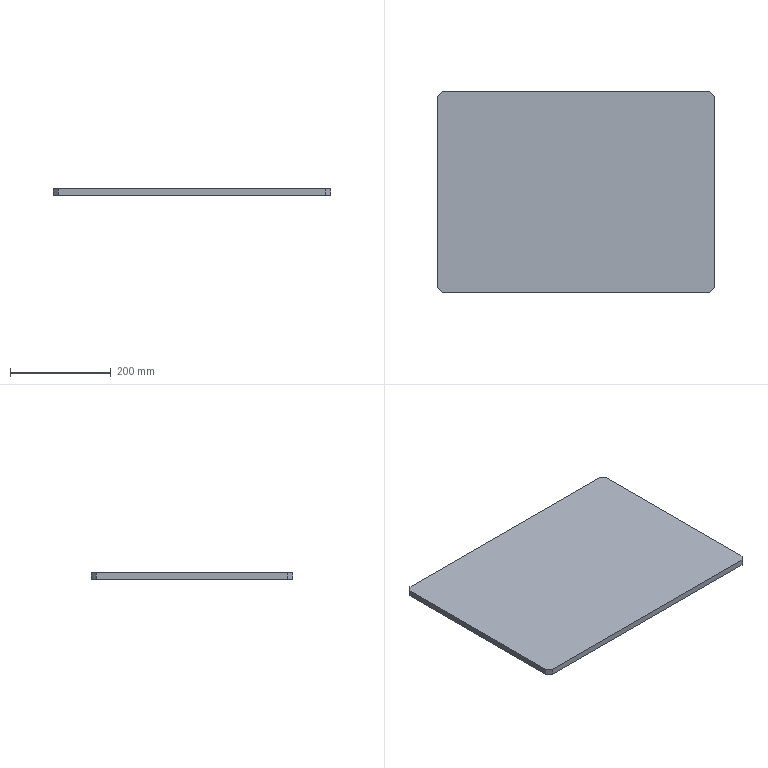Part | NX | features BREP 1 | 1 solid | 10 faces | box 550 x 400 x 12 mm | volume 2637600 mm3 | plane 10
STEP:
#1=CARTESIAN_POINT('',(308.,-205.,0.));
#2=VERTEX_POINT('',#1);
#3=CARTESIAN_POINT('',(308.,175.,0.));
#4=VERTEX_POINT('',#3);
#5=CARTESIAN_POINT('',(308.,-150.,0.));
#6=DIRECTION('',(0.,1.,0.));
#7=VECTOR('',#6,1000.);
#8=LINE('',#5,#7);
#9=EDGE_CURVE('',#2,#4,#8,.T.);
#10=ORIENTED_EDGE('',*,*,#9,.T.);
#11=CARTESIAN_POINT('',(308.,175.,12.));
#12=VERTEX_POINT('',#11);
#13=CARTESIAN_POINT('',(308.,175.,12.));
#14=DIRECTION('',(0.,0.,1.));
#15=VECTOR('',#14,1000.);
#16=LINE('',#13,#15);
#17=EDGE_CURVE('',#4,#12,#16,.T.);
#18=ORIENTED_EDGE('',*,*,#17,.T.);
#19=CARTESIAN_POINT('',(308.,-205.,12.));
#20=VERTEX_POINT('',#19);
#21=CARTESIAN_POINT('',(308.,-150.,12.));
#22=DIRECTION('',(0.,1.,0.));
#23=VECTOR('',#22,1000.);
#24=LINE('',#21,#23);
#25=EDGE_CURVE('',#20,#12,#24,.T.);
#26=ORIENTED_EDGE('',*,*,#25,.F.);
#27=CARTESIAN_POINT('',(308.,-205.,12.));
#28=DIRECTION('',(0.,0.,-1.));
#29=VECTOR('',#28,1000.);
#30=LINE('',#27,#29);
#31=EDGE_CURVE('',#20,#2,#30,.T.);
#32=ORIENTED_EDGE('',*,*,#31,.T.);
#33=EDGE_LOOP('',(#10,#18,#26,#32));
#34=FACE_BOUND('',#33,.T.);
#35=CARTESIAN_POINT('',(308.,-150.,12.));
#36=DIRECTION('',(-1.,0.,0.));
#37=DIRECTION('',(0.,0.,1.));
#38=AXIS2_PLACEMENT_3D('',#35,#36,#37);
#39=PLANE('',#38);
#40=ADVANCED_FACE('',(#34),#39,.F.);
#41=CARTESIAN_POINT('',(298.,185.,0.));
#42=VERTEX_POINT('',#41);
#43=CARTESIAN_POINT('',(-232.,185.,0.));
#44=VERTEX_POINT('',#43);
#45=CARTESIAN_POINT('',(-150.,185.,0.));
#46=DIRECTION('',(-1.,0.,0.));
#47=VECTOR('',#46,1000.);
#48=LINE('',#45,#47);
#49=EDGE_CURVE('',#42,#44,#48,.T.);
#50=ORIENTED_EDGE('',*,*,#49,.T.);
#51=CARTESIAN_POINT('',(-232.,185.,12.));
#52=VERTEX_POINT('',#51);
#53=CARTESIAN_POINT('',(-232.,185.,12.));
#54=DIRECTION('',(0.,0.,1.));
#55=VECTOR('',#54,1000.);
#56=LINE('',#53,#55);
#57=EDGE_CURVE('',#44,#52,#56,.T.);
#58=ORIENTED_EDGE('',*,*,#57,.T.);
#59=CARTESIAN_POINT('',(298.,185.,12.));
#60=VERTEX_POINT('',#59);
#61=CARTESIAN_POINT('',(-150.,185.,12.));
#62=DIRECTION('',(-1.,0.,0.));
#63=VECTOR('',#62,1000.);
#64=LINE('',#61,#63);
#65=EDGE_CURVE('',#60,#52,#64,.T.);
#66=ORIENTED_EDGE('',*,*,#65,.F.);
#67=CARTESIAN_POINT('',(298.,185.,12.));
#68=DIRECTION('',(0.,0.,-1.));
#69=VECTOR('',#68,1000.);
#70=LINE('',#67,#69);
#71=EDGE_CURVE('',#60,#42,#70,.T.);
#72=ORIENTED_EDGE('',*,*,#71,.T.);
#73=EDGE_LOOP('',(#50,#58,#66,#72));
#74=FACE_BOUND('',#73,.T.);
#75=CARTESIAN_POINT('',(-150.,185.,12.));
#76=DIRECTION('',(0.,-1.,0.));
#77=DIRECTION('',(0.,0.,-1.));
#78=AXIS2_PLACEMENT_3D('',#75,#76,#77);
#79=PLANE('',#78);
#80=ADVANCED_FACE('',(#74),#79,.F.);
#81=CARTESIAN_POINT('',(-242.,175.,12.));
#82=VERTEX_POINT('',#81);
#83=CARTESIAN_POINT('',(-242.,-205.,12.));
#84=VERTEX_POINT('',#83);
#85=CARTESIAN_POINT('',(-242.,-150.,12.));
#86=DIRECTION('',(0.,-1.,0.));
#87=VECTOR('',#86,1000.);
#88=LINE('',#85,#87);
#89=EDGE_CURVE('',#82,#84,#88,.T.);
#90=ORIENTED_EDGE('',*,*,#89,.F.);
#91=CARTESIAN_POINT('',(-242.,175.,0.));
#92=VERTEX_POINT('',#91);
#93=CARTESIAN_POINT('',(-242.,175.,12.));
#94=DIRECTION('',(0.,0.,-1.));
#95=VECTOR('',#94,1000.);
#96=LINE('',#93,#95);
#97=EDGE_CURVE('',#82,#92,#96,.T.);
#98=ORIENTED_EDGE('',*,*,#97,.T.);
#99=CARTESIAN_POINT('',(-242.,-205.,0.));
#100=VERTEX_POINT('',#99);
#101=CARTESIAN_POINT('',(-242.,-150.,0.));
#102=DIRECTION('',(0.,-1.,0.));
#103=VECTOR('',#102,1000.);
#104=LINE('',#101,#103);
#105=EDGE_CURVE('',#92,#100,#104,.T.);
#106=ORIENTED_EDGE('',*,*,#105,.T.);
#107=CARTESIAN_POINT('',(-242.,-205.,12.));
#108=DIRECTION('',(0.,0.,1.));
#109=VECTOR('',#108,1000.);
#110=LINE('',#107,#109);
#111=EDGE_CURVE('',#100,#84,#110,.T.);
#112=ORIENTED_EDGE('',*,*,#111,.T.);
#113=EDGE_LOOP('',(#90,#98,#106,#112));
#114=FACE_BOUND('',#113,.T.);
#115=CARTESIAN_POINT('',(-242.,-150.,12.));
#116=DIRECTION('',(1.,0.,0.));
#117=DIRECTION('',(0.,1.,0.));
#118=AXIS2_PLACEMENT_3D('',#115,#116,#117);
#119=PLANE('',#118);
#120=ADVANCED_FACE('',(#114),#119,.F.);
#121=CARTESIAN_POINT('',(-232.,-215.,0.));
#122=VERTEX_POINT('',#121);
#123=CARTESIAN_POINT('',(298.,-215.,0.));
#124=VERTEX_POINT('',#123);
#125=CARTESIAN_POINT('',(-150.,-215.,0.));
#126=DIRECTION('',(1.,0.,0.));
#127=VECTOR('',#126,1000.);
#128=LINE('',#125,#127);
#129=EDGE_CURVE('',#122,#124,#128,.T.);
#130=ORIENTED_EDGE('',*,*,#129,.T.);
#131=CARTESIAN_POINT('',(298.,-215.,12.));
#132=VERTEX_POINT('',#131);
#133=CARTESIAN_POINT('',(298.,-215.,12.));
#134=DIRECTION('',(0.,0.,1.));
#135=VECTOR('',#134,1000.);
#136=LINE('',#133,#135);
#137=EDGE_CURVE('',#124,#132,#136,.T.);
#138=ORIENTED_EDGE('',*,*,#137,.T.);
#139=CARTESIAN_POINT('',(-232.,-215.,12.));
#140=VERTEX_POINT('',#139);
#141=CARTESIAN_POINT('',(-150.,-215.,12.));
#142=DIRECTION('',(1.,0.,0.));
#143=VECTOR('',#142,1000.);
#144=LINE('',#141,#143);
#145=EDGE_CURVE('',#140,#132,#144,.T.);
#146=ORIENTED_EDGE('',*,*,#145,.F.);
#147=CARTESIAN_POINT('',(-232.,-215.,12.));
#148=DIRECTION('',(0.,0.,-1.));
#149=VECTOR('',#148,1000.);
#150=LINE('',#147,#149);
#151=EDGE_CURVE('',#140,#122,#150,.T.);
#152=ORIENTED_EDGE('',*,*,#151,.T.);
#153=EDGE_LOOP('',(#130,#138,#146,#152));
#154=FACE_BOUND('',#153,.T.);
#155=CARTESIAN_POINT('',(-150.,-215.,12.));
#156=DIRECTION('',(0.,1.,0.));
#157=DIRECTION('',(1.,0.,0.));
#158=AXIS2_PLACEMENT_3D('',#155,#156,#157);
#159=PLANE('',#158);
#160=ADVANCED_FACE('',(#154),#159,.F.);
#161=ORIENTED_EDGE('',*,*,#65,.T.);
#162=CARTESIAN_POINT('',(-242.,175.,12.));
#163=DIRECTION('',(-0.7071,-0.7071,0.));
#164=VECTOR('',#163,1000.);
#165=LINE('',#162,#164);
#166=EDGE_CURVE('',#52,#82,#165,.T.);
#167=ORIENTED_EDGE('',*,*,#166,.T.);
#168=ORIENTED_EDGE('',*,*,#89,.T.);
#169=CARTESIAN_POINT('',(-232.,-215.,12.));
#170=DIRECTION('',(0.7071,-0.7071,0.));
#171=VECTOR('',#170,1000.);
#172=LINE('',#169,#171);
#173=EDGE_CURVE('',#84,#140,#172,.T.);
#174=ORIENTED_EDGE('',*,*,#173,.T.);
#175=ORIENTED_EDGE('',*,*,#145,.T.);
#176=CARTESIAN_POINT('',(308.,-205.,12.));
#177=DIRECTION('',(0.7071,0.7071,0.));
#178=VECTOR('',#177,1000.);
#179=LINE('',#176,#178);
#180=EDGE_CURVE('',#132,#20,#179,.T.);
#181=ORIENTED_EDGE('',*,*,#180,.T.);
#182=ORIENTED_EDGE('',*,*,#25,.T.);
#183=CARTESIAN_POINT('',(298.,185.,12.));
#184=DIRECTION('',(-0.7071,0.7071,0.));
#185=VECTOR('',#184,1000.);
#186=LINE('',#183,#185);
#187=EDGE_CURVE('',#12,#60,#186,.T.);
#188=ORIENTED_EDGE('',*,*,#187,.T.);
#189=EDGE_LOOP('',(#161,#167,#168,#174,#175,#181,#182,#188));
#190=FACE_BOUND('',#189,.T.);
#191=CARTESIAN_POINT('',(0.,0.,12.));
#192=DIRECTION('',(0.,0.,-1.));
#193=DIRECTION('',(0.,-1.,0.));
#194=AXIS2_PLACEMENT_3D('',#191,#192,#193);
#195=PLANE('',#194);
#196=ADVANCED_FACE('',(#190),#195,.F.);
#197=ORIENTED_EDGE('',*,*,#105,.F.);
#198=CARTESIAN_POINT('',(-237.,180.,0.));
#199=DIRECTION('',(0.7071,0.7071,0.));
#200=VECTOR('',#199,1000.);
#201=LINE('',#198,#200);
#202=EDGE_CURVE('',#92,#44,#201,.T.);
#203=ORIENTED_EDGE('',*,*,#202,.T.);
#204=ORIENTED_EDGE('',*,*,#49,.F.);
#205=CARTESIAN_POINT('',(303.,180.,0.));
#206=DIRECTION('',(0.7071,-0.7071,0.));
#207=VECTOR('',#206,1000.);
#208=LINE('',#205,#207);
#209=EDGE_CURVE('',#42,#4,#208,.T.);
#210=ORIENTED_EDGE('',*,*,#209,.T.);
#211=ORIENTED_EDGE('',*,*,#9,.F.);
#212=CARTESIAN_POINT('',(303.,-210.,0.));
#213=DIRECTION('',(-0.7071,-0.7071,0.));
#214=VECTOR('',#213,1000.);
#215=LINE('',#212,#214);
#216=EDGE_CURVE('',#2,#124,#215,.T.);
#217=ORIENTED_EDGE('',*,*,#216,.T.);
#218=ORIENTED_EDGE('',*,*,#129,.F.);
#219=CARTESIAN_POINT('',(-237.,-210.,0.));
#220=DIRECTION('',(-0.7071,0.7071,0.));
#221=VECTOR('',#220,1000.);
#222=LINE('',#219,#221);
#223=EDGE_CURVE('',#122,#100,#222,.T.);
#224=ORIENTED_EDGE('',*,*,#223,.T.);
#225=EDGE_LOOP('',(#197,#203,#204,#210,#211,#217,#218,#224));
#226=FACE_BOUND('',#225,.T.);
#227=CARTESIAN_POINT('',(0.,0.,0.));
#228=DIRECTION('',(0.,0.,-1.));
#229=DIRECTION('',(0.,-1.,0.));
#230=AXIS2_PLACEMENT_3D('',#227,#228,#229);
#231=PLANE('',#230);
#232=ADVANCED_FACE('',(#226),#231,.T.);
#233=ORIENTED_EDGE('',*,*,#166,.F.);
#234=ORIENTED_EDGE('',*,*,#57,.F.);
#235=ORIENTED_EDGE('',*,*,#202,.F.);
#236=ORIENTED_EDGE('',*,*,#97,.F.);
#237=EDGE_LOOP('',(#233,#234,#235,#236));
#238=FACE_BOUND('',#237,.T.);
#239=CARTESIAN_POINT('',(-242.,175.,12.));
#240=DIRECTION('',(0.7071,-0.7071,0.));
#241=DIRECTION('',(0.,0.,-1.));
#242=AXIS2_PLACEMENT_3D('',#239,#240,#241);
#243=PLANE('',#242);
#244=ADVANCED_FACE('',(#238),#243,.F.);
#245=ORIENTED_EDGE('',*,*,#187,.F.);
#246=ORIENTED_EDGE('',*,*,#17,.F.);
#247=ORIENTED_EDGE('',*,*,#209,.F.);
#248=ORIENTED_EDGE('',*,*,#71,.F.);
#249=EDGE_LOOP('',(#245,#246,#247,#248));
#250=FACE_BOUND('',#249,.T.);
#251=CARTESIAN_POINT('',(298.,185.,12.));
#252=DIRECTION('',(-0.7071,-0.7071,0.));
#253=DIRECTION('',(-0.7071,0.7071,0.));
#254=AXIS2_PLACEMENT_3D('',#251,#252,#253);
#255=PLANE('',#254);
#256=ADVANCED_FACE('',(#250),#255,.F.);
#257=ORIENTED_EDGE('',*,*,#180,.F.);
#258=ORIENTED_EDGE('',*,*,#137,.F.);
#259=ORIENTED_EDGE('',*,*,#216,.F.);
#260=ORIENTED_EDGE('',*,*,#31,.F.);
#261=EDGE_LOOP('',(#257,#258,#259,#260));
#262=FACE_BOUND('',#261,.T.);
#263=CARTESIAN_POINT('',(308.,-205.,12.));
#264=DIRECTION('',(-0.7071,0.7071,0.));
#265=DIRECTION('',(0.,0.,1.));
#266=AXIS2_PLACEMENT_3D('',#263,#264,#265);
#267=PLANE('',#266);
#268=ADVANCED_FACE('',(#262),#267,.F.);
#269=ORIENTED_EDGE('',*,*,#173,.F.);
#270=ORIENTED_EDGE('',*,*,#111,.F.);
#271=ORIENTED_EDGE('',*,*,#223,.F.);
#272=ORIENTED_EDGE('',*,*,#151,.F.);
#273=EDGE_LOOP('',(#269,#270,#271,#272));
#274=FACE_BOUND('',#273,.T.);
#275=CARTESIAN_POINT('',(-232.,-215.,12.));
#276=DIRECTION('',(0.7071,0.7071,0.));
#277=DIRECTION('',(0.,0.,-1.));
#278=AXIS2_PLACEMENT_3D('',#275,#276,#277);
#279=PLANE('',#278);
#280=ADVANCED_FACE('',(#274),#279,.F.);
#281=CLOSED_SHELL('',(#40,#80,#120,#160,#196,#232,#244,#256,#268,#280));
#282=MANIFOLD_SOLID_BREP('',#281);
#283=(LENGTH_UNIT()NAMED_UNIT(*)SI_UNIT(.MILLI.,.METRE.));
#284=UNCERTAINTY_MEASURE_WITH_UNIT(LENGTH_MEASURE(0.00001),#283,'','');
#285=(NAMED_UNIT(*)PLANE_ANGLE_UNIT()SI_UNIT($,.RADIAN.));
#286=(NAMED_UNIT(*)SI_UNIT($,.STERADIAN.)SOLID_ANGLE_UNIT());
#287=(GEOMETRIC_REPRESENTATION_CONTEXT(3)GLOBAL_UNCERTAINTY_ASSIGNED_CONTEXT((#284))GLOBAL_UNIT_ASSIGNED_CONTEXT((#283,#285,#286))REPRESENTATION_CONTEXT('',''));
#288=ADVANCED_BREP_SHAPE_REPRESENTATION('',(#282),#287);